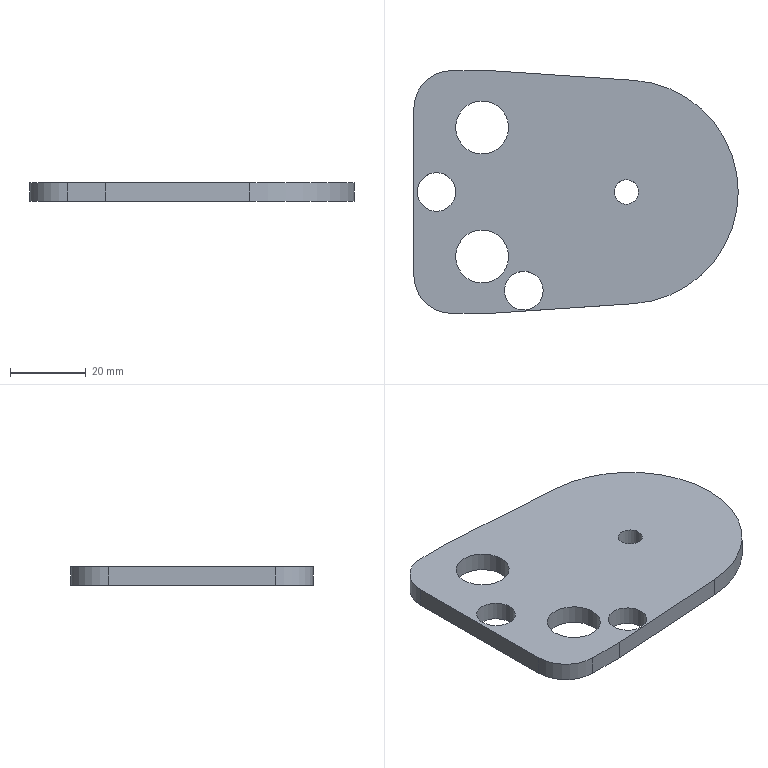Part | NX | features solid 2 | 1 solid | 15 faces | box 85.5 x 64 x 5 mm | volume 21586 mm3 | cylinder 8 | plane 7 | commonest cylinder face diameters 10.2 x2 14 x2 20 x2 6.4 x1 59 x1
STEP:
#1=CARTESIAN_POINT('',(49.,13.006,47.));
#2=VERTEX_POINT('',#1);
#3=CARTESIAN_POINT('',(39.,23.006,47.));
#4=VERTEX_POINT('',#3);
#5=CARTESIAN_POINT('',(49.,23.006,47.));
#6=DIRECTION('',(0.,0.,-1.));
#7=DIRECTION('',(-1.,0.,0.));
#8=AXIS2_PLACEMENT_3D('',#5,#6,#7);
#9=CIRCLE('',#8,10.);
#10=EDGE_CURVE('',#2,#4,#9,.T.);
#11=ORIENTED_EDGE('',*,*,#10,.F.);
#12=CARTESIAN_POINT('',(49.,13.006,52.));
#13=VERTEX_POINT('',#12);
#14=CARTESIAN_POINT('',(49.,13.006,52.));
#15=DIRECTION('',(0.,0.,-1.));
#16=VECTOR('',#15,1000.);
#17=LINE('',#14,#16);
#18=EDGE_CURVE('',#13,#2,#17,.T.);
#19=ORIENTED_EDGE('',*,*,#18,.F.);
#20=CARTESIAN_POINT('',(39.,23.006,52.));
#21=VERTEX_POINT('',#20);
#22=CARTESIAN_POINT('',(49.,23.006,52.));
#23=DIRECTION('',(0.,0.,-1.));
#24=DIRECTION('',(-1.,0.,0.));
#25=AXIS2_PLACEMENT_3D('',#22,#23,#24);
#26=CIRCLE('',#25,10.);
#27=EDGE_CURVE('',#13,#21,#26,.T.);
#28=ORIENTED_EDGE('',*,*,#27,.T.);
#29=CARTESIAN_POINT('',(39.,23.006,52.));
#30=DIRECTION('',(0.,0.,-1.));
#31=VECTOR('',#30,1000.);
#32=LINE('',#29,#31);
#33=EDGE_CURVE('',#21,#4,#32,.T.);
#34=ORIENTED_EDGE('',*,*,#33,.T.);
#35=EDGE_LOOP('',(#11,#19,#28,#34));
#36=FACE_BOUND('',#35,.T.);
#37=CARTESIAN_POINT('',(49.,23.006,52.));
#38=DIRECTION('',(0.,0.,-1.));
#39=DIRECTION('',(-1.,0.,0.));
#40=AXIS2_PLACEMENT_3D('',#37,#38,#39);
#41=CYLINDRICAL_SURFACE('',#40,10.);
#42=ADVANCED_FACE('',(#36),#41,.T.);
#43=CARTESIAN_POINT('',(39.,67.006,47.));
#44=VERTEX_POINT('',#43);
#45=CARTESIAN_POINT('',(39.,67.006,47.));
#46=DIRECTION('',(0.,-1.,0.));
#47=VECTOR('',#46,1000.);
#48=LINE('',#45,#47);
#49=EDGE_CURVE('',#44,#4,#48,.T.);
#50=ORIENTED_EDGE('',*,*,#49,.T.);
#51=ORIENTED_EDGE('',*,*,#33,.F.);
#52=CARTESIAN_POINT('',(39.,67.006,52.));
#53=VERTEX_POINT('',#52);
#54=CARTESIAN_POINT('',(39.,67.006,52.));
#55=DIRECTION('',(0.,-1.,0.));
#56=VECTOR('',#55,1000.);
#57=LINE('',#54,#56);
#58=EDGE_CURVE('',#53,#21,#57,.T.);
#59=ORIENTED_EDGE('',*,*,#58,.F.);
#60=CARTESIAN_POINT('',(39.,67.006,52.));
#61=DIRECTION('',(0.,0.,-1.));
#62=VECTOR('',#61,1000.);
#63=LINE('',#60,#62);
#64=EDGE_CURVE('',#53,#44,#63,.T.);
#65=ORIENTED_EDGE('',*,*,#64,.T.);
#66=EDGE_LOOP('',(#50,#51,#59,#65));
#67=FACE_BOUND('',#66,.T.);
#68=CARTESIAN_POINT('',(39.,67.006,52.));
#69=DIRECTION('',(1.,0.,0.));
#70=DIRECTION('',(0.,1.,0.));
#71=AXIS2_PLACEMENT_3D('',#68,#69,#70);
#72=PLANE('',#71);
#73=ADVANCED_FACE('',(#67),#72,.F.);
#74=CARTESIAN_POINT('',(49.,77.006,47.));
#75=VERTEX_POINT('',#74);
#76=CARTESIAN_POINT('',(49.,67.006,47.));
#77=DIRECTION('',(0.,0.,-1.));
#78=DIRECTION('',(-1.,0.,0.));
#79=AXIS2_PLACEMENT_3D('',#76,#77,#78);
#80=CIRCLE('',#79,10.);
#81=EDGE_CURVE('',#44,#75,#80,.T.);
#82=ORIENTED_EDGE('',*,*,#81,.F.);
#83=ORIENTED_EDGE('',*,*,#64,.F.);
#84=CARTESIAN_POINT('',(49.,77.006,52.));
#85=VERTEX_POINT('',#84);
#86=CARTESIAN_POINT('',(49.,67.006,52.));
#87=DIRECTION('',(0.,0.,-1.));
#88=DIRECTION('',(-1.,0.,0.));
#89=AXIS2_PLACEMENT_3D('',#86,#87,#88);
#90=CIRCLE('',#89,10.);
#91=EDGE_CURVE('',#53,#85,#90,.T.);
#92=ORIENTED_EDGE('',*,*,#91,.T.);
#93=CARTESIAN_POINT('',(49.,77.006,52.));
#94=DIRECTION('',(0.,0.,-1.));
#95=VECTOR('',#94,1000.);
#96=LINE('',#93,#95);
#97=EDGE_CURVE('',#85,#75,#96,.T.);
#98=ORIENTED_EDGE('',*,*,#97,.T.);
#99=EDGE_LOOP('',(#82,#83,#92,#98));
#100=FACE_BOUND('',#99,.T.);
#101=CARTESIAN_POINT('',(49.,67.006,52.));
#102=DIRECTION('',(0.,0.,-1.));
#103=DIRECTION('',(-1.,0.,0.));
#104=AXIS2_PLACEMENT_3D('',#101,#102,#103);
#105=CYLINDRICAL_SURFACE('',#104,10.);
#106=ADVANCED_FACE('',(#100),#105,.T.);
#107=CARTESIAN_POINT('',(59.,77.006,47.));
#108=VERTEX_POINT('',#107);
#109=CARTESIAN_POINT('',(59.,77.006,47.));
#110=DIRECTION('',(-1.,0.,0.));
#111=VECTOR('',#110,1000.);
#112=LINE('',#109,#111);
#113=EDGE_CURVE('',#108,#75,#112,.T.);
#114=ORIENTED_EDGE('',*,*,#113,.T.);
#115=ORIENTED_EDGE('',*,*,#97,.F.);
#116=CARTESIAN_POINT('',(59.,77.006,52.));
#117=VERTEX_POINT('',#116);
#118=CARTESIAN_POINT('',(59.,77.006,52.));
#119=DIRECTION('',(-1.,0.,0.));
#120=VECTOR('',#119,1000.);
#121=LINE('',#118,#120);
#122=EDGE_CURVE('',#117,#85,#121,.T.);
#123=ORIENTED_EDGE('',*,*,#122,.F.);
#124=CARTESIAN_POINT('',(59.,77.006,52.));
#125=DIRECTION('',(0.,0.,-1.));
#126=VECTOR('',#125,1000.);
#127=LINE('',#124,#126);
#128=EDGE_CURVE('',#117,#108,#127,.T.);
#129=ORIENTED_EDGE('',*,*,#128,.T.);
#130=EDGE_LOOP('',(#114,#115,#123,#129));
#131=FACE_BOUND('',#130,.T.);
#132=CARTESIAN_POINT('',(59.,77.006,52.));
#133=DIRECTION('',(0.,-1.,0.));
#134=DIRECTION('',(0.,0.,-1.));
#135=AXIS2_PLACEMENT_3D('',#132,#133,#134);
#136=PLANE('',#135);
#137=ADVANCED_FACE('',(#131),#136,.F.);
#138=CARTESIAN_POINT('',(96.989,74.439,47.));
#139=VERTEX_POINT('',#138);
#140=CARTESIAN_POINT('',(96.989,74.439,47.));
#141=DIRECTION('',(-0.9977,0.06742,0.));
#142=VECTOR('',#141,1000.);
#143=LINE('',#140,#142);
#144=EDGE_CURVE('',#139,#108,#143,.T.);
#145=ORIENTED_EDGE('',*,*,#144,.T.);
#146=ORIENTED_EDGE('',*,*,#128,.F.);
#147=CARTESIAN_POINT('',(96.989,74.439,52.));
#148=VERTEX_POINT('',#147);
#149=CARTESIAN_POINT('',(96.989,74.439,52.));
#150=DIRECTION('',(-0.9977,0.06742,0.));
#151=VECTOR('',#150,1000.);
#152=LINE('',#149,#151);
#153=EDGE_CURVE('',#148,#117,#152,.T.);
#154=ORIENTED_EDGE('',*,*,#153,.F.);
#155=CARTESIAN_POINT('',(96.989,74.439,52.));
#156=DIRECTION('',(0.,0.,-1.));
#157=VECTOR('',#156,1000.);
#158=LINE('',#155,#157);
#159=EDGE_CURVE('',#148,#139,#158,.T.);
#160=ORIENTED_EDGE('',*,*,#159,.T.);
#161=EDGE_LOOP('',(#145,#146,#154,#160));
#162=FACE_BOUND('',#161,.T.);
#163=CARTESIAN_POINT('',(96.989,74.439,52.));
#164=DIRECTION('',(-0.06742,-0.9977,0.));
#165=DIRECTION('',(0.9977,-0.06742,0.));
#166=AXIS2_PLACEMENT_3D('',#163,#164,#165);
#167=PLANE('',#166);
#168=ADVANCED_FACE('',(#162),#167,.F.);
#169=CARTESIAN_POINT('',(96.989,15.574,47.));
#170=VERTEX_POINT('',#169);
#171=CARTESIAN_POINT('',(95.,45.006,47.));
#172=DIRECTION('',(0.,0.,-1.));
#173=DIRECTION('',(-1.,0.,0.));
#174=AXIS2_PLACEMENT_3D('',#171,#172,#173);
#175=CIRCLE('',#174,29.5);
#176=EDGE_CURVE('',#139,#170,#175,.T.);
#177=ORIENTED_EDGE('',*,*,#176,.F.);
#178=ORIENTED_EDGE('',*,*,#159,.F.);
#179=CARTESIAN_POINT('',(96.989,15.574,52.));
#180=VERTEX_POINT('',#179);
#181=CARTESIAN_POINT('',(95.,45.006,52.));
#182=DIRECTION('',(0.,0.,-1.));
#183=DIRECTION('',(-1.,0.,0.));
#184=AXIS2_PLACEMENT_3D('',#181,#182,#183);
#185=CIRCLE('',#184,29.5);
#186=EDGE_CURVE('',#148,#180,#185,.T.);
#187=ORIENTED_EDGE('',*,*,#186,.T.);
#188=CARTESIAN_POINT('',(96.989,15.574,52.));
#189=DIRECTION('',(0.,0.,-1.));
#190=VECTOR('',#189,1000.);
#191=LINE('',#188,#190);
#192=EDGE_CURVE('',#180,#170,#191,.T.);
#193=ORIENTED_EDGE('',*,*,#192,.T.);
#194=EDGE_LOOP('',(#177,#178,#187,#193));
#195=FACE_BOUND('',#194,.T.);
#196=CARTESIAN_POINT('',(95.,45.006,52.));
#197=DIRECTION('',(0.,0.,-1.));
#198=DIRECTION('',(-1.,0.,0.));
#199=AXIS2_PLACEMENT_3D('',#196,#197,#198);
#200=CYLINDRICAL_SURFACE('',#199,29.5);
#201=ADVANCED_FACE('',(#195),#200,.T.);
#202=CARTESIAN_POINT('',(59.,13.006,47.));
#203=VERTEX_POINT('',#202);
#204=CARTESIAN_POINT('',(96.989,15.574,47.));
#205=DIRECTION('',(-0.9977,-0.06742,0.));
#206=VECTOR('',#205,1000.);
#207=LINE('',#204,#206);
#208=EDGE_CURVE('',#170,#203,#207,.T.);
#209=ORIENTED_EDGE('',*,*,#208,.F.);
#210=ORIENTED_EDGE('',*,*,#192,.F.);
#211=CARTESIAN_POINT('',(59.,13.006,52.));
#212=VERTEX_POINT('',#211);
#213=CARTESIAN_POINT('',(96.989,15.574,52.));
#214=DIRECTION('',(-0.9977,-0.06742,0.));
#215=VECTOR('',#214,1000.);
#216=LINE('',#213,#215);
#217=EDGE_CURVE('',#180,#212,#216,.T.);
#218=ORIENTED_EDGE('',*,*,#217,.T.);
#219=CARTESIAN_POINT('',(59.,13.006,52.));
#220=DIRECTION('',(0.,0.,-1.));
#221=VECTOR('',#220,1000.);
#222=LINE('',#219,#221);
#223=EDGE_CURVE('',#212,#203,#222,.T.);
#224=ORIENTED_EDGE('',*,*,#223,.T.);
#225=EDGE_LOOP('',(#209,#210,#218,#224));
#226=FACE_BOUND('',#225,.T.);
#227=CARTESIAN_POINT('',(96.989,15.574,52.));
#228=DIRECTION('',(0.06742,-0.9977,0.));
#229=DIRECTION('',(0.9977,0.06742,0.));
#230=AXIS2_PLACEMENT_3D('',#227,#228,#229);
#231=PLANE('',#230);
#232=ADVANCED_FACE('',(#226),#231,.T.);
#233=CARTESIAN_POINT('',(59.,13.006,47.));
#234=DIRECTION('',(-1.,0.,0.));
#235=VECTOR('',#234,1000.);
#236=LINE('',#233,#235);
#237=EDGE_CURVE('',#203,#2,#236,.T.);
#238=ORIENTED_EDGE('',*,*,#237,.F.);
#239=ORIENTED_EDGE('',*,*,#223,.F.);
#240=CARTESIAN_POINT('',(59.,13.006,52.));
#241=DIRECTION('',(-1.,0.,0.));
#242=VECTOR('',#241,1000.);
#243=LINE('',#240,#242);
#244=EDGE_CURVE('',#212,#13,#243,.T.);
#245=ORIENTED_EDGE('',*,*,#244,.T.);
#246=ORIENTED_EDGE('',*,*,#18,.T.);
#247=EDGE_LOOP('',(#238,#239,#245,#246));
#248=FACE_BOUND('',#247,.T.);
#249=CARTESIAN_POINT('',(59.,13.006,52.));
#250=DIRECTION('',(0.,-1.,0.));
#251=DIRECTION('',(1.,0.,0.));
#252=AXIS2_PLACEMENT_3D('',#249,#250,#251);
#253=PLANE('',#252);
#254=ADVANCED_FACE('',(#248),#253,.T.);
#255=CARTESIAN_POINT('',(50.,62.006,52.));
#256=VERTEX_POINT('',#255);
#257=CARTESIAN_POINT('',(57.,62.006,52.));
#258=DIRECTION('',(0.,0.,-1.));
#259=DIRECTION('',(-1.,0.,0.));
#260=AXIS2_PLACEMENT_3D('',#257,#258,#259);
#261=CIRCLE('',#260,7.);
#262=EDGE_CURVE('',#256,#256,#261,.T.);
#263=ORIENTED_EDGE('',*,*,#262,.T.);
#264=EDGE_LOOP('',(#263));
#265=FACE_BOUND('',#264,.T.);
#266=CARTESIAN_POINT('',(50.,28.006,52.));
#267=VERTEX_POINT('',#266);
#268=CARTESIAN_POINT('',(57.,28.006,52.));
#269=DIRECTION('',(0.,0.,-1.));
#270=DIRECTION('',(-1.,0.,0.));
#271=AXIS2_PLACEMENT_3D('',#268,#269,#270);
#272=CIRCLE('',#271,7.);
#273=EDGE_CURVE('',#267,#267,#272,.T.);
#274=ORIENTED_EDGE('',*,*,#273,.T.);
#275=EDGE_LOOP('',(#274));
#276=FACE_BOUND('',#275,.T.);
#277=CARTESIAN_POINT('',(91.8,45.006,52.));
#278=VERTEX_POINT('',#277);
#279=CARTESIAN_POINT('',(95.,45.006,52.));
#280=DIRECTION('',(0.,0.,-1.));
#281=DIRECTION('',(-1.,0.,0.));
#282=AXIS2_PLACEMENT_3D('',#279,#280,#281);
#283=CIRCLE('',#282,3.2);
#284=EDGE_CURVE('',#278,#278,#283,.T.);
#285=ORIENTED_EDGE('',*,*,#284,.T.);
#286=EDGE_LOOP('',(#285));
#287=FACE_BOUND('',#286,.T.);
#288=CARTESIAN_POINT('',(62.9,19.006,52.));
#289=VERTEX_POINT('',#288);
#290=CARTESIAN_POINT('',(68.,19.006,52.));
#291=DIRECTION('',(0.,0.,-1.));
#292=DIRECTION('',(-1.,0.,0.));
#293=AXIS2_PLACEMENT_3D('',#290,#291,#292);
#294=CIRCLE('',#293,5.1);
#295=EDGE_CURVE('',#289,#289,#294,.T.);
#296=ORIENTED_EDGE('',*,*,#295,.T.);
#297=EDGE_LOOP('',(#296));
#298=FACE_BOUND('',#297,.T.);
#299=CARTESIAN_POINT('',(39.9,45.006,52.));
#300=VERTEX_POINT('',#299);
#301=CARTESIAN_POINT('',(45.,45.006,52.));
#302=DIRECTION('',(0.,0.,-1.));
#303=DIRECTION('',(-1.,0.,0.));
#304=AXIS2_PLACEMENT_3D('',#301,#302,#303);
#305=CIRCLE('',#304,5.1);
#306=EDGE_CURVE('',#300,#300,#305,.T.);
#307=ORIENTED_EDGE('',*,*,#306,.T.);
#308=EDGE_LOOP('',(#307));
#309=FACE_BOUND('',#308,.T.);
#310=ORIENTED_EDGE('',*,*,#27,.F.);
#311=ORIENTED_EDGE('',*,*,#244,.F.);
#312=ORIENTED_EDGE('',*,*,#217,.F.);
#313=ORIENTED_EDGE('',*,*,#186,.F.);
#314=ORIENTED_EDGE('',*,*,#153,.T.);
#315=ORIENTED_EDGE('',*,*,#122,.T.);
#316=ORIENTED_EDGE('',*,*,#91,.F.);
#317=ORIENTED_EDGE('',*,*,#58,.T.);
#318=EDGE_LOOP('',(#310,#311,#312,#313,#314,#315,#316,#317));
#319=FACE_BOUND('',#318,.T.);
#320=CARTESIAN_POINT('',(49.,23.006,52.));
#321=DIRECTION('',(0.,0.,-1.));
#322=DIRECTION('',(-1.,0.,0.));
#323=AXIS2_PLACEMENT_3D('',#320,#321,#322);
#324=PLANE('',#323);
#325=ADVANCED_FACE('',(#265,#276,#287,#298,#309,#319),#324,.F.);
#326=CARTESIAN_POINT('',(50.,62.006,47.));
#327=VERTEX_POINT('',#326);
#328=CARTESIAN_POINT('',(57.,62.006,47.));
#329=DIRECTION('',(0.,0.,-1.));
#330=DIRECTION('',(-1.,0.,0.));
#331=AXIS2_PLACEMENT_3D('',#328,#329,#330);
#332=CIRCLE('',#331,7.);
#333=EDGE_CURVE('',#327,#327,#332,.T.);
#334=ORIENTED_EDGE('',*,*,#333,.F.);
#335=EDGE_LOOP('',(#334));
#336=FACE_BOUND('',#335,.T.);
#337=CARTESIAN_POINT('',(50.,28.006,47.));
#338=VERTEX_POINT('',#337);
#339=CARTESIAN_POINT('',(57.,28.006,47.));
#340=DIRECTION('',(0.,0.,-1.));
#341=DIRECTION('',(-1.,0.,0.));
#342=AXIS2_PLACEMENT_3D('',#339,#340,#341);
#343=CIRCLE('',#342,7.);
#344=EDGE_CURVE('',#338,#338,#343,.T.);
#345=ORIENTED_EDGE('',*,*,#344,.F.);
#346=EDGE_LOOP('',(#345));
#347=FACE_BOUND('',#346,.T.);
#348=CARTESIAN_POINT('',(91.8,45.006,47.));
#349=VERTEX_POINT('',#348);
#350=CARTESIAN_POINT('',(95.,45.006,47.));
#351=DIRECTION('',(0.,0.,-1.));
#352=DIRECTION('',(-1.,0.,0.));
#353=AXIS2_PLACEMENT_3D('',#350,#351,#352);
#354=CIRCLE('',#353,3.2);
#355=EDGE_CURVE('',#349,#349,#354,.T.);
#356=ORIENTED_EDGE('',*,*,#355,.F.);
#357=EDGE_LOOP('',(#356));
#358=FACE_BOUND('',#357,.T.);
#359=CARTESIAN_POINT('',(62.9,19.006,47.));
#360=VERTEX_POINT('',#359);
#361=CARTESIAN_POINT('',(68.,19.006,47.));
#362=DIRECTION('',(0.,0.,-1.));
#363=DIRECTION('',(-1.,0.,0.));
#364=AXIS2_PLACEMENT_3D('',#361,#362,#363);
#365=CIRCLE('',#364,5.1);
#366=EDGE_CURVE('',#360,#360,#365,.T.);
#367=ORIENTED_EDGE('',*,*,#366,.F.);
#368=EDGE_LOOP('',(#367));
#369=FACE_BOUND('',#368,.T.);
#370=CARTESIAN_POINT('',(39.9,45.006,47.));
#371=VERTEX_POINT('',#370);
#372=CARTESIAN_POINT('',(45.,45.006,47.));
#373=DIRECTION('',(0.,0.,-1.));
#374=DIRECTION('',(-1.,0.,0.));
#375=AXIS2_PLACEMENT_3D('',#372,#373,#374);
#376=CIRCLE('',#375,5.1);
#377=EDGE_CURVE('',#371,#371,#376,.T.);
#378=ORIENTED_EDGE('',*,*,#377,.F.);
#379=EDGE_LOOP('',(#378));
#380=FACE_BOUND('',#379,.T.);
#381=ORIENTED_EDGE('',*,*,#10,.T.);
#382=ORIENTED_EDGE('',*,*,#49,.F.);
#383=ORIENTED_EDGE('',*,*,#81,.T.);
#384=ORIENTED_EDGE('',*,*,#113,.F.);
#385=ORIENTED_EDGE('',*,*,#144,.F.);
#386=ORIENTED_EDGE('',*,*,#176,.T.);
#387=ORIENTED_EDGE('',*,*,#208,.T.);
#388=ORIENTED_EDGE('',*,*,#237,.T.);
#389=EDGE_LOOP('',(#381,#382,#383,#384,#385,#386,#387,#388));
#390=FACE_BOUND('',#389,.T.);
#391=CARTESIAN_POINT('',(49.,23.006,47.));
#392=DIRECTION('',(0.,0.,-1.));
#393=DIRECTION('',(-1.,0.,0.));
#394=AXIS2_PLACEMENT_3D('',#391,#392,#393);
#395=PLANE('',#394);
#396=ADVANCED_FACE('',(#336,#347,#358,#369,#380,#390),#395,.T.);
#397=ORIENTED_EDGE('',*,*,#377,.T.);
#398=EDGE_LOOP('',(#397));
#399=FACE_BOUND('',#398,.T.);
#400=ORIENTED_EDGE('',*,*,#306,.F.);
#401=EDGE_LOOP('',(#400));
#402=FACE_BOUND('',#401,.T.);
#403=CARTESIAN_POINT('',(45.,45.006,52.));
#404=DIRECTION('',(0.,0.,-1.));
#405=DIRECTION('',(-1.,0.,0.));
#406=AXIS2_PLACEMENT_3D('',#403,#404,#405);
#407=CYLINDRICAL_SURFACE('',#406,5.1);
#408=ADVANCED_FACE('',(#399,#402),#407,.F.);
#409=ORIENTED_EDGE('',*,*,#366,.T.);
#410=EDGE_LOOP('',(#409));
#411=FACE_BOUND('',#410,.T.);
#412=ORIENTED_EDGE('',*,*,#295,.F.);
#413=EDGE_LOOP('',(#412));
#414=FACE_BOUND('',#413,.T.);
#415=CARTESIAN_POINT('',(68.,19.006,52.));
#416=DIRECTION('',(0.,0.,-1.));
#417=DIRECTION('',(-1.,0.,0.));
#418=AXIS2_PLACEMENT_3D('',#415,#416,#417);
#419=CYLINDRICAL_SURFACE('',#418,5.1);
#420=ADVANCED_FACE('',(#411,#414),#419,.F.);
#421=ORIENTED_EDGE('',*,*,#355,.T.);
#422=EDGE_LOOP('',(#421));
#423=FACE_BOUND('',#422,.T.);
#424=ORIENTED_EDGE('',*,*,#284,.F.);
#425=EDGE_LOOP('',(#424));
#426=FACE_BOUND('',#425,.T.);
#427=CARTESIAN_POINT('',(95.,45.006,52.));
#428=DIRECTION('',(0.,0.,-1.));
#429=DIRECTION('',(-1.,0.,0.));
#430=AXIS2_PLACEMENT_3D('',#427,#428,#429);
#431=CYLINDRICAL_SURFACE('',#430,3.2);
#432=ADVANCED_FACE('',(#423,#426),#431,.F.);
#433=ORIENTED_EDGE('',*,*,#344,.T.);
#434=EDGE_LOOP('',(#433));
#435=FACE_BOUND('',#434,.T.);
#436=ORIENTED_EDGE('',*,*,#273,.F.);
#437=EDGE_LOOP('',(#436));
#438=FACE_BOUND('',#437,.T.);
#439=CARTESIAN_POINT('',(57.,28.006,52.));
#440=DIRECTION('',(0.,0.,-1.));
#441=DIRECTION('',(-1.,0.,0.));
#442=AXIS2_PLACEMENT_3D('',#439,#440,#441);
#443=CYLINDRICAL_SURFACE('',#442,7.);
#444=ADVANCED_FACE('',(#435,#438),#443,.F.);
#445=ORIENTED_EDGE('',*,*,#333,.T.);
#446=EDGE_LOOP('',(#445));
#447=FACE_BOUND('',#446,.T.);
#448=ORIENTED_EDGE('',*,*,#262,.F.);
#449=EDGE_LOOP('',(#448));
#450=FACE_BOUND('',#449,.T.);
#451=CARTESIAN_POINT('',(57.,62.006,52.));
#452=DIRECTION('',(0.,0.,-1.));
#453=DIRECTION('',(-1.,0.,0.));
#454=AXIS2_PLACEMENT_3D('',#451,#452,#453);
#455=CYLINDRICAL_SURFACE('',#454,7.);
#456=ADVANCED_FACE('',(#447,#450),#455,.F.);
#457=CLOSED_SHELL('',(#42,#73,#106,#137,#168,#201,#232,#254,#325,#396,#408,#420,#432,#444,#456));
#458=MANIFOLD_SOLID_BREP('',#457);
#459=(LENGTH_UNIT()NAMED_UNIT(*)SI_UNIT(.MILLI.,.METRE.));
#460=UNCERTAINTY_MEASURE_WITH_UNIT(LENGTH_MEASURE(0.00001),#459,'','');
#461=(NAMED_UNIT(*)PLANE_ANGLE_UNIT()SI_UNIT($,.RADIAN.));
#462=(NAMED_UNIT(*)SI_UNIT($,.STERADIAN.)SOLID_ANGLE_UNIT());
#463=(GEOMETRIC_REPRESENTATION_CONTEXT(3)GLOBAL_UNCERTAINTY_ASSIGNED_CONTEXT((#460))GLOBAL_UNIT_ASSIGNED_CONTEXT((#459,#461,#462))REPRESENTATION_CONTEXT('',''));
#464=ADVANCED_BREP_SHAPE_REPRESENTATION('',(#458),#463);